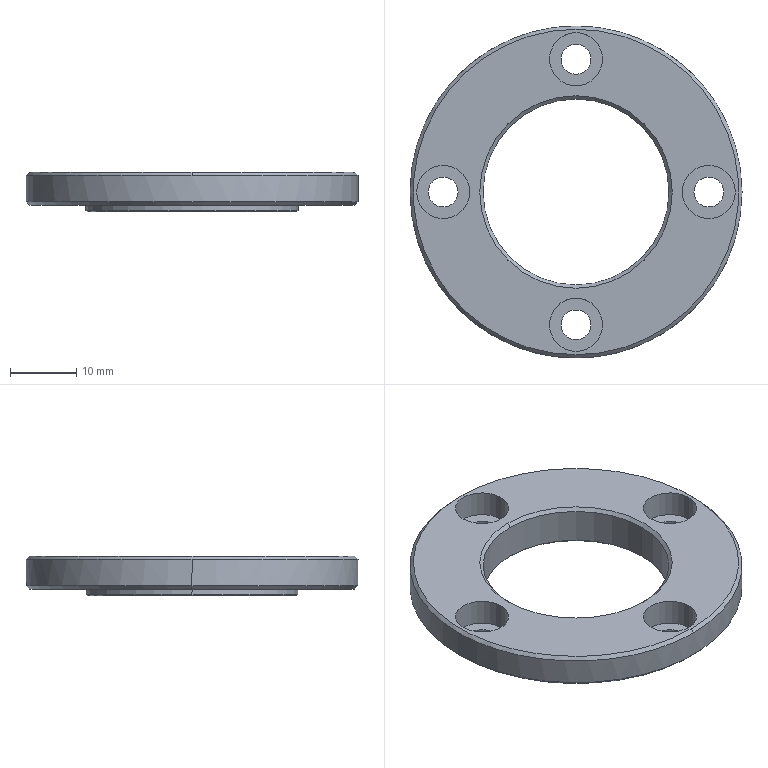Part | STEP file | locating sleeve 2 | 1 solid | 39 faces | box 50 x 50 x 6 mm | volume 6005 mm3 | cylinder 22 | cone 10 | plane 7 | commonest cylinder face diameters 4.5 x8 8 x8 28 x2 32 x2 50 x2